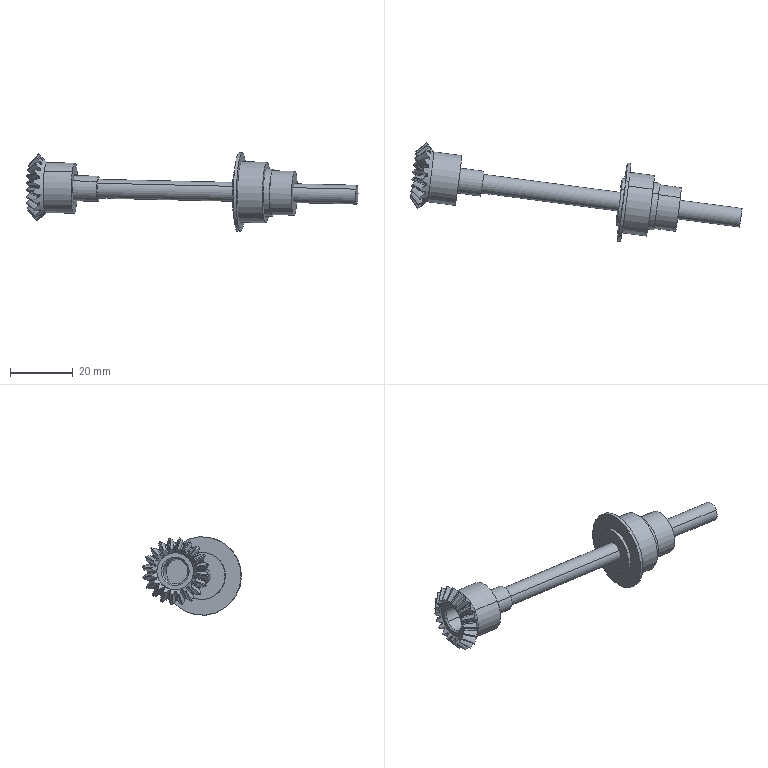Part | SolidWorks | 4 solids | 167 faces | box 105.649 x 31.478 x 25.016 mm | volume 9209 mm3 | spline 100 | cone 28 | cylinder 26 | plane 13 | commonest cylinder face diameters 8 x4 11.8 x4 15 x4 3 x2 5 x2 6 x2